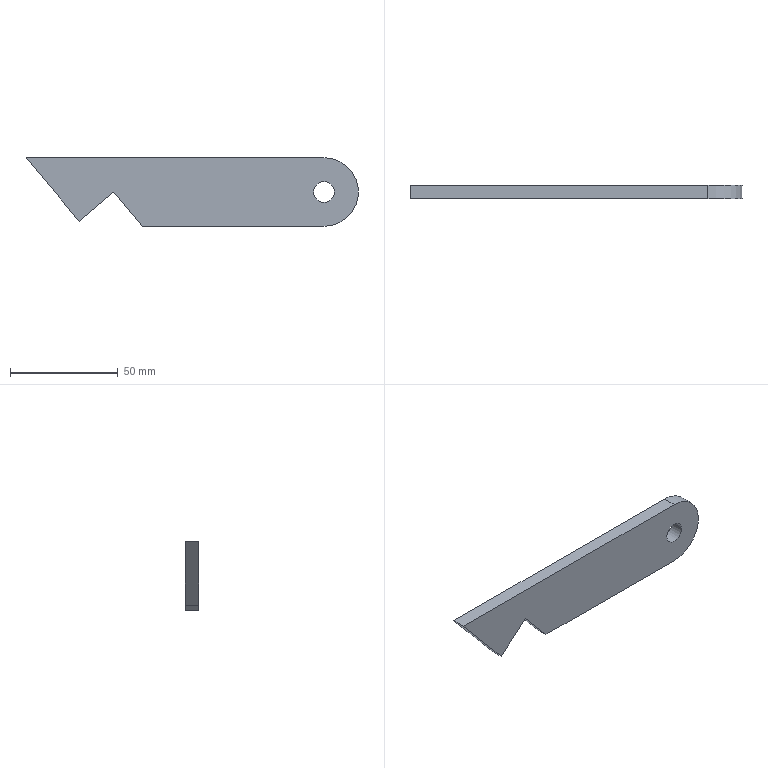Part | NX | features BREP 1 | 1 solid | 10 faces | box 153.924 x 6.35 x 31.75 mm | volume 25607 mm3 | plane 7 | cylinder 3 | commonest cylinder face diameters 9.652 x2 31.75 x1
STEP:
#1=CARTESIAN_POINT('',(45.561,0.,0.));
#2=VERTEX_POINT('',#1);
#3=CARTESIAN_POINT('',(29.473,0.,-13.499));
#4=VERTEX_POINT('',#3);
#5=CARTESIAN_POINT('',(45.561,0.,0.));
#6=DIRECTION('',(-0.766,0.,-0.6428));
#7=VECTOR('',#6,1000.);
#8=LINE('',#5,#7);
#9=EDGE_CURVE('',#2,#4,#8,.T.);
#10=ORIENTED_EDGE('',*,*,#9,.T.);
#11=CARTESIAN_POINT('',(4.826,0.,15.875));
#12=VERTEX_POINT('',#11);
#13=CARTESIAN_POINT('',(29.473,0.,-13.499));
#14=DIRECTION('',(-0.6428,0.,0.766));
#15=VECTOR('',#14,1000.);
#16=LINE('',#13,#15);
#17=EDGE_CURVE('',#4,#12,#16,.T.);
#18=ORIENTED_EDGE('',*,*,#17,.T.);
#19=CARTESIAN_POINT('',(142.875,0.,15.875));
#20=VERTEX_POINT('',#19);
#21=CARTESIAN_POINT('',(4.826,0.,15.875));
#22=DIRECTION('',(1.,0.,0.));
#23=VECTOR('',#22,1000.);
#24=LINE('',#21,#23);
#25=EDGE_CURVE('',#12,#20,#24,.T.);
#26=ORIENTED_EDGE('',*,*,#25,.T.);
#27=CARTESIAN_POINT('',(142.875,0.,-15.875));
#28=VERTEX_POINT('',#27);
#29=CARTESIAN_POINT('',(142.875,0.,0.));
#30=DIRECTION('',(0.,1.,0.));
#31=DIRECTION('',(0.,0.,1.));
#32=AXIS2_PLACEMENT_3D('',#29,#30,#31);
#33=CIRCLE('',#32,15.875);
#34=EDGE_CURVE('',#20,#28,#33,.T.);
#35=ORIENTED_EDGE('',*,*,#34,.T.);
#36=CARTESIAN_POINT('',(58.881,0.,-15.875));
#37=VERTEX_POINT('',#36);
#38=CARTESIAN_POINT('',(142.875,0.,-15.875));
#39=DIRECTION('',(-1.,0.,0.));
#40=VECTOR('',#39,1000.);
#41=LINE('',#38,#40);
#42=EDGE_CURVE('',#28,#37,#41,.T.);
#43=ORIENTED_EDGE('',*,*,#42,.T.);
#44=CARTESIAN_POINT('',(58.881,0.,-15.875));
#45=DIRECTION('',(-0.6428,0.,0.766));
#46=VECTOR('',#45,1000.);
#47=LINE('',#44,#46);
#48=EDGE_CURVE('',#37,#2,#47,.T.);
#49=ORIENTED_EDGE('',*,*,#48,.T.);
#50=EDGE_LOOP('',(#10,#18,#26,#35,#43,#49));
#51=FACE_BOUND('',#50,.T.);
#52=CARTESIAN_POINT('',(147.701,0.,0.));
#53=VERTEX_POINT('',#52);
#54=CARTESIAN_POINT('',(138.049,0.,0.));
#55=VERTEX_POINT('',#54);
#56=CARTESIAN_POINT('',(142.875,0.,0.));
#57=DIRECTION('',(0.,1.,0.));
#58=DIRECTION('',(1.,0.,0.));
#59=AXIS2_PLACEMENT_3D('',#56,#57,#58);
#60=CIRCLE('',#59,4.826);
#61=EDGE_CURVE('',#53,#55,#60,.T.);
#62=ORIENTED_EDGE('',*,*,#61,.F.);
#63=CARTESIAN_POINT('',(142.875,0.,0.));
#64=DIRECTION('',(0.,1.,0.));
#65=DIRECTION('',(-1.,0.,0.));
#66=AXIS2_PLACEMENT_3D('',#63,#64,#65);
#67=CIRCLE('',#66,4.826);
#68=EDGE_CURVE('',#55,#53,#67,.T.);
#69=ORIENTED_EDGE('',*,*,#68,.F.);
#70=EDGE_LOOP('',(#62,#69));
#71=FACE_BOUND('',#70,.T.);
#72=CARTESIAN_POINT('',(0.,0.,0.));
#73=DIRECTION('',(0.,1.,0.));
#74=DIRECTION('',(1.,0.,0.));
#75=AXIS2_PLACEMENT_3D('',#72,#73,#74);
#76=PLANE('',#75);
#77=ADVANCED_FACE('',(#51,#71),#76,.T.);
#78=CARTESIAN_POINT('',(147.701,-6.35,0.));
#79=VERTEX_POINT('',#78);
#80=CARTESIAN_POINT('',(147.701,0.,0.));
#81=DIRECTION('',(0.,-1.,0.));
#82=VECTOR('',#81,1000.);
#83=LINE('',#80,#82);
#84=EDGE_CURVE('',#79,#53,#83,.F.);
#85=ORIENTED_EDGE('',*,*,#84,.F.);
#86=CARTESIAN_POINT('',(138.049,-6.35,0.));
#87=VERTEX_POINT('',#86);
#88=CARTESIAN_POINT('',(142.875,-6.35,0.));
#89=DIRECTION('',(0.,1.,0.));
#90=DIRECTION('',(-1.,0.,0.));
#91=AXIS2_PLACEMENT_3D('',#88,#89,#90);
#92=CIRCLE('',#91,4.826);
#93=EDGE_CURVE('',#87,#79,#92,.T.);
#94=ORIENTED_EDGE('',*,*,#93,.F.);
#95=CARTESIAN_POINT('',(138.049,0.,0.));
#96=DIRECTION('',(0.,-1.,0.));
#97=VECTOR('',#96,1000.);
#98=LINE('',#95,#97);
#99=EDGE_CURVE('',#87,#55,#98,.F.);
#100=ORIENTED_EDGE('',*,*,#99,.T.);
#101=ORIENTED_EDGE('',*,*,#68,.T.);
#102=EDGE_LOOP('',(#85,#94,#100,#101));
#103=FACE_BOUND('',#102,.T.);
#104=CARTESIAN_POINT('',(142.875,-3.175,0.));
#105=DIRECTION('',(0.,1.,0.));
#106=DIRECTION('',(-1.,0.,0.));
#107=AXIS2_PLACEMENT_3D('',#104,#105,#106);
#108=CYLINDRICAL_SURFACE('',#107,4.826);
#109=ADVANCED_FACE('',(#103),#108,.F.);
#110=ORIENTED_EDGE('',*,*,#99,.F.);
#111=CARTESIAN_POINT('',(142.875,-6.35,0.));
#112=DIRECTION('',(0.,1.,0.));
#113=DIRECTION('',(1.,0.,0.));
#114=AXIS2_PLACEMENT_3D('',#111,#112,#113);
#115=CIRCLE('',#114,4.826);
#116=EDGE_CURVE('',#79,#87,#115,.T.);
#117=ORIENTED_EDGE('',*,*,#116,.F.);
#118=ORIENTED_EDGE('',*,*,#84,.T.);
#119=ORIENTED_EDGE('',*,*,#61,.T.);
#120=EDGE_LOOP('',(#110,#117,#118,#119));
#121=FACE_BOUND('',#120,.T.);
#122=CARTESIAN_POINT('',(142.875,-3.175,0.));
#123=DIRECTION('',(0.,1.,0.));
#124=DIRECTION('',(1.,0.,0.));
#125=AXIS2_PLACEMENT_3D('',#122,#123,#124);
#126=CYLINDRICAL_SURFACE('',#125,4.826);
#127=ADVANCED_FACE('',(#121),#126,.F.);
#128=CARTESIAN_POINT('',(142.875,-6.35,-15.875));
#129=VERTEX_POINT('',#128);
#130=CARTESIAN_POINT('',(58.881,-6.35,-15.875));
#131=VERTEX_POINT('',#130);
#132=CARTESIAN_POINT('',(142.875,-6.35,-15.875));
#133=DIRECTION('',(-1.,0.,0.));
#134=VECTOR('',#133,1000.);
#135=LINE('',#132,#134);
#136=EDGE_CURVE('',#129,#131,#135,.T.);
#137=ORIENTED_EDGE('',*,*,#136,.F.);
#138=CARTESIAN_POINT('',(142.875,-6.35,15.875));
#139=VERTEX_POINT('',#138);
#140=CARTESIAN_POINT('',(142.875,-6.35,0.));
#141=DIRECTION('',(0.,1.,0.));
#142=DIRECTION('',(0.,0.,1.));
#143=AXIS2_PLACEMENT_3D('',#140,#141,#142);
#144=CIRCLE('',#143,15.875);
#145=EDGE_CURVE('',#139,#129,#144,.T.);
#146=ORIENTED_EDGE('',*,*,#145,.F.);
#147=CARTESIAN_POINT('',(4.826,-6.35,15.875));
#148=VERTEX_POINT('',#147);
#149=CARTESIAN_POINT('',(4.826,-6.35,15.875));
#150=DIRECTION('',(1.,0.,0.));
#151=VECTOR('',#150,1000.);
#152=LINE('',#149,#151);
#153=EDGE_CURVE('',#148,#139,#152,.T.);
#154=ORIENTED_EDGE('',*,*,#153,.F.);
#155=CARTESIAN_POINT('',(29.473,-6.35,-13.499));
#156=VERTEX_POINT('',#155);
#157=CARTESIAN_POINT('',(29.473,-6.35,-13.499));
#158=DIRECTION('',(-0.6428,0.,0.766));
#159=VECTOR('',#158,1000.);
#160=LINE('',#157,#159);
#161=EDGE_CURVE('',#156,#148,#160,.T.);
#162=ORIENTED_EDGE('',*,*,#161,.F.);
#163=CARTESIAN_POINT('',(45.561,-6.35,0.));
#164=VERTEX_POINT('',#163);
#165=CARTESIAN_POINT('',(45.561,-6.35,0.));
#166=DIRECTION('',(-0.766,0.,-0.6428));
#167=VECTOR('',#166,1000.);
#168=LINE('',#165,#167);
#169=EDGE_CURVE('',#164,#156,#168,.T.);
#170=ORIENTED_EDGE('',*,*,#169,.F.);
#171=CARTESIAN_POINT('',(58.881,-6.35,-15.875));
#172=DIRECTION('',(-0.6428,0.,0.766));
#173=VECTOR('',#172,1000.);
#174=LINE('',#171,#173);
#175=EDGE_CURVE('',#131,#164,#174,.T.);
#176=ORIENTED_EDGE('',*,*,#175,.F.);
#177=EDGE_LOOP('',(#137,#146,#154,#162,#170,#176));
#178=FACE_BOUND('',#177,.T.);
#179=ORIENTED_EDGE('',*,*,#116,.T.);
#180=ORIENTED_EDGE('',*,*,#93,.T.);
#181=EDGE_LOOP('',(#179,#180));
#182=FACE_BOUND('',#181,.T.);
#183=CARTESIAN_POINT('',(0.,-6.35,0.));
#184=DIRECTION('',(0.,1.,0.));
#185=DIRECTION('',(1.,0.,0.));
#186=AXIS2_PLACEMENT_3D('',#183,#184,#185);
#187=PLANE('',#186);
#188=ADVANCED_FACE('',(#178,#182),#187,.F.);
#189=CARTESIAN_POINT('',(58.881,0.,-15.875));
#190=DIRECTION('',(0.,-1.,0.));
#191=VECTOR('',#190,1000.);
#192=LINE('',#189,#191);
#193=EDGE_CURVE('',#37,#131,#192,.T.);
#194=ORIENTED_EDGE('',*,*,#193,.T.);
#195=ORIENTED_EDGE('',*,*,#175,.T.);
#196=CARTESIAN_POINT('',(45.561,0.,0.));
#197=DIRECTION('',(0.,-1.,0.));
#198=VECTOR('',#197,1000.);
#199=LINE('',#196,#198);
#200=EDGE_CURVE('',#2,#164,#199,.T.);
#201=ORIENTED_EDGE('',*,*,#200,.F.);
#202=ORIENTED_EDGE('',*,*,#48,.F.);
#203=EDGE_LOOP('',(#194,#195,#201,#202));
#204=FACE_BOUND('',#203,.T.);
#205=CARTESIAN_POINT('',(52.221,-3.175,-7.938));
#206=DIRECTION('',(-0.766,0.,-0.6428));
#207=DIRECTION('',(-0.6428,0.,0.766));
#208=AXIS2_PLACEMENT_3D('',#205,#206,#207);
#209=PLANE('',#208);
#210=ADVANCED_FACE('',(#204),#209,.T.);
#211=ORIENTED_EDGE('',*,*,#200,.T.);
#212=ORIENTED_EDGE('',*,*,#169,.T.);
#213=CARTESIAN_POINT('',(29.473,0.,-13.499));
#214=DIRECTION('',(0.,-1.,0.));
#215=VECTOR('',#214,1000.);
#216=LINE('',#213,#215);
#217=EDGE_CURVE('',#4,#156,#216,.T.);
#218=ORIENTED_EDGE('',*,*,#217,.F.);
#219=ORIENTED_EDGE('',*,*,#9,.F.);
#220=EDGE_LOOP('',(#211,#212,#218,#219));
#221=FACE_BOUND('',#220,.T.);
#222=CARTESIAN_POINT('',(37.517,-3.175,-6.749));
#223=DIRECTION('',(0.6428,0.,-0.766));
#224=DIRECTION('',(0.,-1.,0.));
#225=AXIS2_PLACEMENT_3D('',#222,#223,#224);
#226=PLANE('',#225);
#227=ADVANCED_FACE('',(#221),#226,.T.);
#228=ORIENTED_EDGE('',*,*,#217,.T.);
#229=ORIENTED_EDGE('',*,*,#161,.T.);
#230=CARTESIAN_POINT('',(4.826,0.,15.875));
#231=DIRECTION('',(0.,-1.,0.));
#232=VECTOR('',#231,1000.);
#233=LINE('',#230,#232);
#234=EDGE_CURVE('',#12,#148,#233,.T.);
#235=ORIENTED_EDGE('',*,*,#234,.F.);
#236=ORIENTED_EDGE('',*,*,#17,.F.);
#237=EDGE_LOOP('',(#228,#229,#235,#236));
#238=FACE_BOUND('',#237,.T.);
#239=CARTESIAN_POINT('',(17.15,-3.175,1.188));
#240=DIRECTION('',(-0.766,0.,-0.6428));
#241=DIRECTION('',(-0.6428,0.,0.766));
#242=AXIS2_PLACEMENT_3D('',#239,#240,#241);
#243=PLANE('',#242);
#244=ADVANCED_FACE('',(#238),#243,.T.);
#245=ORIENTED_EDGE('',*,*,#153,.T.);
#246=CARTESIAN_POINT('',(142.875,0.,15.875));
#247=DIRECTION('',(0.,-1.,0.));
#248=VECTOR('',#247,1000.);
#249=LINE('',#246,#248);
#250=EDGE_CURVE('',#20,#139,#249,.T.);
#251=ORIENTED_EDGE('',*,*,#250,.F.);
#252=ORIENTED_EDGE('',*,*,#25,.F.);
#253=ORIENTED_EDGE('',*,*,#234,.T.);
#254=EDGE_LOOP('',(#245,#251,#252,#253));
#255=FACE_BOUND('',#254,.T.);
#256=CARTESIAN_POINT('',(71.438,-3.175,15.875));
#257=DIRECTION('',(0.,0.,1.));
#258=DIRECTION('',(1.,0.,0.));
#259=AXIS2_PLACEMENT_3D('',#256,#257,#258);
#260=PLANE('',#259);
#261=ADVANCED_FACE('',(#255),#260,.T.);
#262=ORIENTED_EDGE('',*,*,#250,.T.);
#263=ORIENTED_EDGE('',*,*,#145,.T.);
#264=CARTESIAN_POINT('',(142.875,0.,-15.875));
#265=DIRECTION('',(0.,-1.,0.));
#266=VECTOR('',#265,1000.);
#267=LINE('',#264,#266);
#268=EDGE_CURVE('',#28,#129,#267,.T.);
#269=ORIENTED_EDGE('',*,*,#268,.F.);
#270=ORIENTED_EDGE('',*,*,#34,.F.);
#271=EDGE_LOOP('',(#262,#263,#269,#270));
#272=FACE_BOUND('',#271,.T.);
#273=CARTESIAN_POINT('',(142.875,-3.175,0.));
#274=DIRECTION('',(0.,1.,0.));
#275=DIRECTION('',(0.,0.,1.));
#276=AXIS2_PLACEMENT_3D('',#273,#274,#275);
#277=CYLINDRICAL_SURFACE('',#276,15.875);
#278=ADVANCED_FACE('',(#272),#277,.T.);
#279=ORIENTED_EDGE('',*,*,#42,.F.);
#280=ORIENTED_EDGE('',*,*,#268,.T.);
#281=ORIENTED_EDGE('',*,*,#136,.T.);
#282=ORIENTED_EDGE('',*,*,#193,.F.);
#283=EDGE_LOOP('',(#279,#280,#281,#282));
#284=FACE_BOUND('',#283,.T.);
#285=CARTESIAN_POINT('',(71.438,-3.175,-15.875));
#286=DIRECTION('',(0.,0.,-1.));
#287=DIRECTION('',(0.,-1.,0.));
#288=AXIS2_PLACEMENT_3D('',#285,#286,#287);
#289=PLANE('',#288);
#290=ADVANCED_FACE('',(#284),#289,.T.);
#291=CLOSED_SHELL('',(#77,#109,#127,#188,#210,#227,#244,#261,#278,#290));
#292=MANIFOLD_SOLID_BREP('',#291);
#293=(LENGTH_UNIT()NAMED_UNIT(*)SI_UNIT(.MILLI.,.METRE.));
#294=UNCERTAINTY_MEASURE_WITH_UNIT(LENGTH_MEASURE(0.00001),#293,'','');
#295=(NAMED_UNIT(*)PLANE_ANGLE_UNIT()SI_UNIT($,.RADIAN.));
#296=(NAMED_UNIT(*)SI_UNIT($,.STERADIAN.)SOLID_ANGLE_UNIT());
#297=(GEOMETRIC_REPRESENTATION_CONTEXT(3)GLOBAL_UNCERTAINTY_ASSIGNED_CONTEXT((#294))GLOBAL_UNIT_ASSIGNED_CONTEXT((#293,#295,#296))REPRESENTATION_CONTEXT('',''));
#298=ADVANCED_BREP_SHAPE_REPRESENTATION('',(#292),#297);